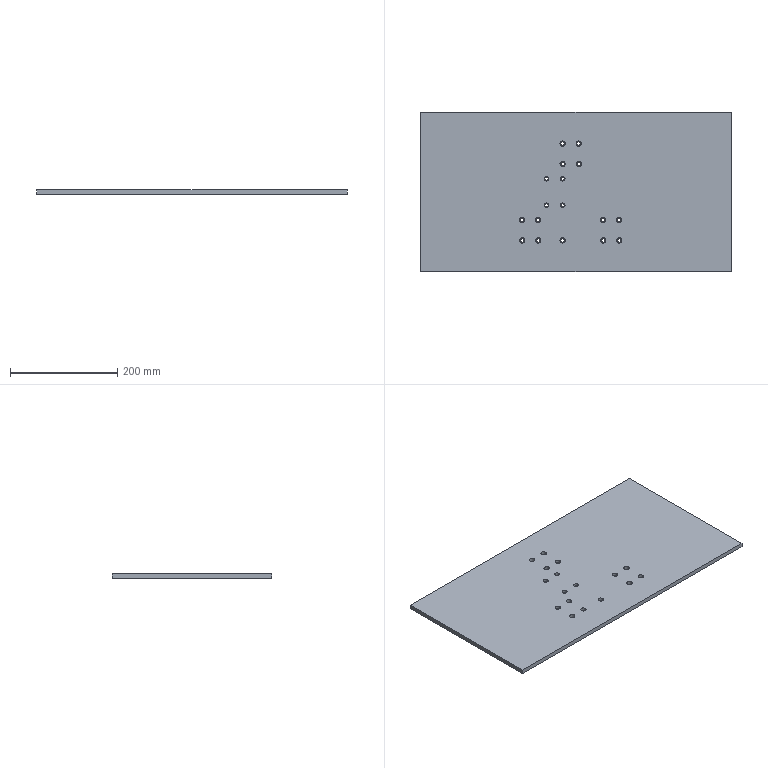Part | 1 solid | 91 faces | box 580 x 297 x 8 mm | volume 1369479 mm3 | cylinder 68 | plane 23 | commonest cylinder face diameters 6.5 x26 10 x26 6 x8 9 x8